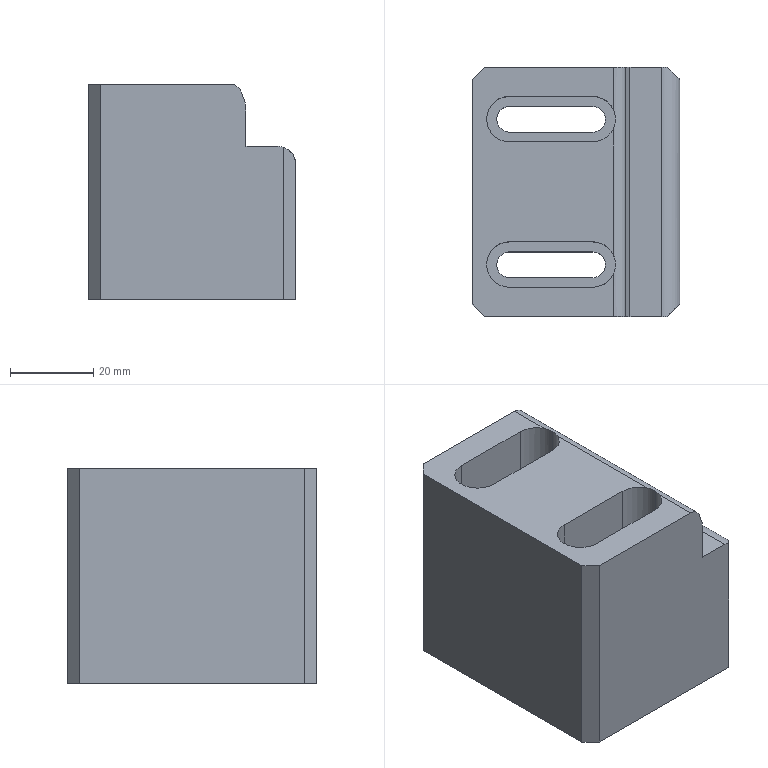Part | SolidWorks | features ICE 3, Chamfer 2, Fillet 2, Extrusion 1 | 1 solid | 38 faces | box 50 x 60 x 52 mm | volume 117515 mm3 | plane 23 | cylinder 15 | commonest cylinder face diameters 6.2 x6 11 x6 6 x2 8.8 x1
STEP:
#1=CARTESIAN_POINT('',(-2.536,-24.104,20.));
#2=VERTEX_POINT('',#1);
#3=CARTESIAN_POINT('',(-8.036,-18.604,20.));
#4=VERTEX_POINT('',#3);
#5=CARTESIAN_POINT('',(-8.036,-24.104,20.));
#6=DIRECTION('',(0.,0.,1.));
#7=DIRECTION('',(1.,0.,0.));
#8=AXIS2_PLACEMENT_3D('',#5,#6,#7);
#9=CIRCLE('',#8,5.5);
#10=EDGE_CURVE('',#2,#4,#9,.T.);
#11=ORIENTED_EDGE('',*,*,#10,.F.);
#12=CARTESIAN_POINT('',(-2.536,-24.104,51.97));
#13=VERTEX_POINT('',#12);
#14=CARTESIAN_POINT('',(-2.536,-24.104,20.));
#15=DIRECTION('',(0.,0.,1.));
#16=VECTOR('',#15,1000.);
#17=LINE('',#14,#16);
#18=EDGE_CURVE('',#2,#13,#17,.T.);
#19=ORIENTED_EDGE('',*,*,#18,.T.);
#20=CARTESIAN_POINT('',(-2.956,-21.995,52.));
#21=VERTEX_POINT('',#20);
#22=CARTESIAN_POINT('',(-2.536,-24.104,51.97));
#23=CARTESIAN_POINT('',(-2.536,-23.745,51.97));
#24=CARTESIAN_POINT('',(-2.57,-23.388,51.976));
#25=CARTESIAN_POINT('',(-2.711,-22.678,51.991));
#26=CARTESIAN_POINT('',(-2.817,-22.33,52.));
#27=CARTESIAN_POINT('',(-2.956,-21.995,52.));
#28=B_SPLINE_CURVE_WITH_KNOTS('',3,(#22,#23,#24,#25,#26,#27),.UNSPECIFIED.,.F.,.F.,(4,2,4),(0.002159,0.003239,0.004318),.UNSPECIFIED.);
#29=EDGE_CURVE('',#13,#21,#28,.T.);
#30=ORIENTED_EDGE('',*,*,#29,.T.);
#31=CARTESIAN_POINT('',(-8.036,-18.604,52.));
#32=VERTEX_POINT('',#31);
#33=CARTESIAN_POINT('',(-8.036,-24.104,52.));
#34=DIRECTION('',(0.,0.,1.));
#35=DIRECTION('',(1.,0.,0.));
#36=AXIS2_PLACEMENT_3D('',#33,#34,#35);
#37=CIRCLE('',#36,5.5);
#38=EDGE_CURVE('',#21,#32,#37,.T.);
#39=ORIENTED_EDGE('',*,*,#38,.T.);
#40=CARTESIAN_POINT('',(-8.036,-18.604,20.));
#41=DIRECTION('',(0.,0.,1.));
#42=VECTOR('',#41,1000.);
#43=LINE('',#40,#42);
#44=EDGE_CURVE('',#4,#32,#43,.T.);
#45=ORIENTED_EDGE('',*,*,#44,.F.);
#46=EDGE_LOOP('',(#11,#19,#30,#39,#45));
#47=FACE_OUTER_BOUND('',#46,.T.);
#48=CARTESIAN_POINT('',(-8.036,-24.104,20.));
#49=DIRECTION('',(0.,0.,1.));
#50=DIRECTION('',(1.,0.,0.));
#51=AXIS2_PLACEMENT_3D('',#48,#49,#50);
#52=CYLINDRICAL_SURFACE('',#51,5.5);
#53=ADVANCED_FACE('',(#47),#52,.F.);
#54=CARTESIAN_POINT('',(-2.536,10.896,20.));
#55=VERTEX_POINT('',#54);
#56=CARTESIAN_POINT('',(-8.036,16.396,20.));
#57=VERTEX_POINT('',#56);
#58=CARTESIAN_POINT('',(-8.036,10.896,20.));
#59=DIRECTION('',(0.,0.,1.));
#60=DIRECTION('',(1.,0.,0.));
#61=AXIS2_PLACEMENT_3D('',#58,#59,#60);
#62=CIRCLE('',#61,5.5);
#63=EDGE_CURVE('',#55,#57,#62,.T.);
#64=ORIENTED_EDGE('',*,*,#63,.F.);
#65=CARTESIAN_POINT('',(-2.536,10.896,51.97));
#66=VERTEX_POINT('',#65);
#67=CARTESIAN_POINT('',(-2.536,10.896,20.));
#68=DIRECTION('',(0.,0.,1.));
#69=VECTOR('',#68,1000.);
#70=LINE('',#67,#69);
#71=EDGE_CURVE('',#55,#66,#70,.T.);
#72=ORIENTED_EDGE('',*,*,#71,.T.);
#73=CARTESIAN_POINT('',(-2.956,13.005,52.));
#74=VERTEX_POINT('',#73);
#75=CARTESIAN_POINT('',(-2.536,10.896,51.97));
#76=CARTESIAN_POINT('',(-2.536,11.255,51.97));
#77=CARTESIAN_POINT('',(-2.57,11.612,51.976));
#78=CARTESIAN_POINT('',(-2.711,12.322,51.991));
#79=CARTESIAN_POINT('',(-2.817,12.67,52.));
#80=CARTESIAN_POINT('',(-2.956,13.005,52.));
#81=B_SPLINE_CURVE_WITH_KNOTS('',3,(#75,#76,#77,#78,#79,#80),.UNSPECIFIED.,.F.,.F.,(4,2,4),(0.002159,0.003239,0.004318),.UNSPECIFIED.);
#82=EDGE_CURVE('',#66,#74,#81,.T.);
#83=ORIENTED_EDGE('',*,*,#82,.T.);
#84=CARTESIAN_POINT('',(-8.036,16.396,52.));
#85=VERTEX_POINT('',#84);
#86=CARTESIAN_POINT('',(-8.036,10.896,52.));
#87=DIRECTION('',(0.,0.,1.));
#88=DIRECTION('',(1.,0.,0.));
#89=AXIS2_PLACEMENT_3D('',#86,#87,#88);
#90=CIRCLE('',#89,5.5);
#91=EDGE_CURVE('',#74,#85,#90,.T.);
#92=ORIENTED_EDGE('',*,*,#91,.T.);
#93=CARTESIAN_POINT('',(-8.036,16.396,20.));
#94=DIRECTION('',(0.,0.,1.));
#95=VECTOR('',#94,1000.);
#96=LINE('',#93,#95);
#97=EDGE_CURVE('',#57,#85,#96,.T.);
#98=ORIENTED_EDGE('',*,*,#97,.F.);
#99=EDGE_LOOP('',(#64,#72,#83,#92,#98));
#100=FACE_OUTER_BOUND('',#99,.T.);
#101=CARTESIAN_POINT('',(-8.036,10.896,20.));
#102=DIRECTION('',(0.,0.,1.));
#103=DIRECTION('',(1.,0.,0.));
#104=AXIS2_PLACEMENT_3D('',#101,#102,#103);
#105=CYLINDRICAL_SURFACE('',#104,5.5);
#106=ADVANCED_FACE('',(#100),#105,.F.);
#107=CARTESIAN_POINT('',(-4.936,10.896,0.));
#108=VERTEX_POINT('',#107);
#109=CARTESIAN_POINT('',(-8.036,13.996,0.));
#110=VERTEX_POINT('',#109);
#111=CARTESIAN_POINT('',(-8.036,10.896,0.));
#112=DIRECTION('',(0.,0.,1.));
#113=DIRECTION('',(1.,0.,0.));
#114=AXIS2_PLACEMENT_3D('',#111,#112,#113);
#115=CIRCLE('',#114,3.1);
#116=EDGE_CURVE('',#108,#110,#115,.T.);
#117=ORIENTED_EDGE('',*,*,#116,.F.);
#118=CARTESIAN_POINT('',(-4.936,10.896,20.));
#119=VERTEX_POINT('',#118);
#120=CARTESIAN_POINT('',(-4.936,10.896,0.));
#121=DIRECTION('',(0.,0.,1.));
#122=VECTOR('',#121,1000.);
#123=LINE('',#120,#122);
#124=EDGE_CURVE('',#108,#119,#123,.T.);
#125=ORIENTED_EDGE('',*,*,#124,.T.);
#126=CARTESIAN_POINT('',(-8.036,13.996,20.));
#127=VERTEX_POINT('',#126);
#128=CARTESIAN_POINT('',(-8.036,10.896,20.));
#129=DIRECTION('',(0.,0.,-1.));
#130=DIRECTION('',(1.,0.,0.));
#131=AXIS2_PLACEMENT_3D('',#128,#129,#130);
#132=CIRCLE('',#131,3.1);
#133=EDGE_CURVE('',#127,#119,#132,.T.);
#134=ORIENTED_EDGE('',*,*,#133,.F.);
#135=CARTESIAN_POINT('',(-8.036,13.996,0.));
#136=DIRECTION('',(0.,0.,1.));
#137=VECTOR('',#136,1000.);
#138=LINE('',#135,#137);
#139=EDGE_CURVE('',#110,#127,#138,.T.);
#140=ORIENTED_EDGE('',*,*,#139,.F.);
#141=EDGE_LOOP('',(#117,#125,#134,#140));
#142=FACE_OUTER_BOUND('',#141,.T.);
#143=CARTESIAN_POINT('',(-8.036,10.896,0.));
#144=DIRECTION('',(0.,0.,1.));
#145=DIRECTION('',(1.,0.,0.));
#146=AXIS2_PLACEMENT_3D('',#143,#144,#145);
#147=CYLINDRICAL_SURFACE('',#146,3.1);
#148=ADVANCED_FACE('',(#142),#147,.F.);
#149=CARTESIAN_POINT('',(-4.936,-24.104,0.));
#150=VERTEX_POINT('',#149);
#151=CARTESIAN_POINT('',(-8.036,-21.004,0.));
#152=VERTEX_POINT('',#151);
#153=CARTESIAN_POINT('',(-8.036,-24.104,0.));
#154=DIRECTION('',(0.,0.,1.));
#155=DIRECTION('',(1.,0.,0.));
#156=AXIS2_PLACEMENT_3D('',#153,#154,#155);
#157=CIRCLE('',#156,3.1);
#158=EDGE_CURVE('',#150,#152,#157,.T.);
#159=ORIENTED_EDGE('',*,*,#158,.F.);
#160=CARTESIAN_POINT('',(-4.936,-24.104,20.));
#161=VERTEX_POINT('',#160);
#162=CARTESIAN_POINT('',(-4.936,-24.104,0.));
#163=DIRECTION('',(0.,0.,1.));
#164=VECTOR('',#163,1000.);
#165=LINE('',#162,#164);
#166=EDGE_CURVE('',#150,#161,#165,.T.);
#167=ORIENTED_EDGE('',*,*,#166,.T.);
#168=CARTESIAN_POINT('',(-8.036,-21.004,20.));
#169=VERTEX_POINT('',#168);
#170=CARTESIAN_POINT('',(-8.036,-24.104,20.));
#171=DIRECTION('',(0.,0.,-1.));
#172=DIRECTION('',(1.,0.,0.));
#173=AXIS2_PLACEMENT_3D('',#170,#171,#172);
#174=CIRCLE('',#173,3.1);
#175=EDGE_CURVE('',#169,#161,#174,.T.);
#176=ORIENTED_EDGE('',*,*,#175,.F.);
#177=CARTESIAN_POINT('',(-8.036,-21.004,0.));
#178=DIRECTION('',(0.,0.,1.));
#179=VECTOR('',#178,1000.);
#180=LINE('',#177,#179);
#181=EDGE_CURVE('',#152,#169,#180,.T.);
#182=ORIENTED_EDGE('',*,*,#181,.F.);
#183=EDGE_LOOP('',(#159,#167,#176,#182));
#184=FACE_OUTER_BOUND('',#183,.T.);
#185=CARTESIAN_POINT('',(-8.036,-24.104,0.));
#186=DIRECTION('',(0.,0.,1.));
#187=DIRECTION('',(1.,0.,0.));
#188=AXIS2_PLACEMENT_3D('',#185,#186,#187);
#189=CYLINDRICAL_SURFACE('',#188,3.1);
#190=ADVANCED_FACE('',(#184),#189,.F.);
#191=CARTESIAN_POINT('',(-28.036,-27.204,20.));
#192=VERTEX_POINT('',#191);
#193=CARTESIAN_POINT('',(-28.036,-21.004,20.));
#194=VERTEX_POINT('',#193);
#195=CARTESIAN_POINT('',(-28.036,-24.104,20.));
#196=DIRECTION('',(0.,0.,-1.));
#197=DIRECTION('',(1.,0.,0.));
#198=AXIS2_PLACEMENT_3D('',#195,#196,#197);
#199=CIRCLE('',#198,3.1);
#200=EDGE_CURVE('',#192,#194,#199,.T.);
#201=ORIENTED_EDGE('',*,*,#200,.F.);
#202=CARTESIAN_POINT('',(-28.036,-27.204,0.));
#203=VERTEX_POINT('',#202);
#204=CARTESIAN_POINT('',(-28.036,-27.204,0.));
#205=DIRECTION('',(0.,0.,1.));
#206=VECTOR('',#205,1000.);
#207=LINE('',#204,#206);
#208=EDGE_CURVE('',#203,#192,#207,.T.);
#209=ORIENTED_EDGE('',*,*,#208,.F.);
#210=CARTESIAN_POINT('',(-28.036,-21.004,0.));
#211=VERTEX_POINT('',#210);
#212=CARTESIAN_POINT('',(-28.036,-24.104,0.));
#213=DIRECTION('',(0.,0.,1.));
#214=DIRECTION('',(1.,0.,0.));
#215=AXIS2_PLACEMENT_3D('',#212,#213,#214);
#216=CIRCLE('',#215,3.1);
#217=EDGE_CURVE('',#211,#203,#216,.T.);
#218=ORIENTED_EDGE('',*,*,#217,.F.);
#219=CARTESIAN_POINT('',(-28.036,-21.004,0.));
#220=DIRECTION('',(0.,0.,1.));
#221=VECTOR('',#220,1000.);
#222=LINE('',#219,#221);
#223=EDGE_CURVE('',#211,#194,#222,.T.);
#224=ORIENTED_EDGE('',*,*,#223,.T.);
#225=EDGE_LOOP('',(#201,#209,#218,#224));
#226=FACE_OUTER_BOUND('',#225,.T.);
#227=CARTESIAN_POINT('',(-28.036,-24.104,0.));
#228=DIRECTION('',(0.,0.,1.));
#229=DIRECTION('',(1.,0.,0.));
#230=AXIS2_PLACEMENT_3D('',#227,#228,#229);
#231=CYLINDRICAL_SURFACE('',#230,3.1);
#232=ADVANCED_FACE('',(#226),#231,.F.);
#233=CARTESIAN_POINT('',(-28.036,-21.004,20.));
#234=DIRECTION('',(1.,0.,0.));
#235=VECTOR('',#234,1000.);
#236=LINE('',#233,#235);
#237=EDGE_CURVE('',#194,#169,#236,.T.);
#238=ORIENTED_EDGE('',*,*,#237,.F.);
#239=ORIENTED_EDGE('',*,*,#223,.F.);
#240=CARTESIAN_POINT('',(-28.036,-21.004,0.));
#241=DIRECTION('',(-1.,0.,0.));
#242=VECTOR('',#241,1000.);
#243=LINE('',#240,#242);
#244=EDGE_CURVE('',#152,#211,#243,.T.);
#245=ORIENTED_EDGE('',*,*,#244,.F.);
#246=ORIENTED_EDGE('',*,*,#181,.T.);
#247=EDGE_LOOP('',(#238,#239,#245,#246));
#248=FACE_OUTER_BOUND('',#247,.T.);
#249=CARTESIAN_POINT('',(-28.036,-21.004,0.));
#250=DIRECTION('',(0.,1.,0.));
#251=DIRECTION('',(-1.,0.,0.));
#252=AXIS2_PLACEMENT_3D('',#249,#250,#251);
#253=PLANE('',#252);
#254=ADVANCED_FACE('',(#248),#253,.F.);
#255=ORIENTED_EDGE('',*,*,#166,.F.);
#256=CARTESIAN_POINT('',(-8.036,-27.204,0.));
#257=VERTEX_POINT('',#256);
#258=CARTESIAN_POINT('',(-8.036,-24.104,0.));
#259=DIRECTION('',(0.,0.,1.));
#260=DIRECTION('',(1.,0.,0.));
#261=AXIS2_PLACEMENT_3D('',#258,#259,#260);
#262=CIRCLE('',#261,3.1);
#263=EDGE_CURVE('',#257,#150,#262,.T.);
#264=ORIENTED_EDGE('',*,*,#263,.F.);
#265=CARTESIAN_POINT('',(-8.036,-27.204,20.));
#266=VERTEX_POINT('',#265);
#267=CARTESIAN_POINT('',(-8.036,-27.204,0.));
#268=DIRECTION('',(0.,0.,1.));
#269=VECTOR('',#268,1000.);
#270=LINE('',#267,#269);
#271=EDGE_CURVE('',#257,#266,#270,.T.);
#272=ORIENTED_EDGE('',*,*,#271,.T.);
#273=CARTESIAN_POINT('',(-8.036,-24.104,20.));
#274=DIRECTION('',(0.,0.,-1.));
#275=DIRECTION('',(1.,0.,0.));
#276=AXIS2_PLACEMENT_3D('',#273,#274,#275);
#277=CIRCLE('',#276,3.1);
#278=EDGE_CURVE('',#161,#266,#277,.T.);
#279=ORIENTED_EDGE('',*,*,#278,.F.);
#280=EDGE_LOOP('',(#255,#264,#272,#279));
#281=FACE_OUTER_BOUND('',#280,.T.);
#282=CARTESIAN_POINT('',(-8.036,-24.104,0.));
#283=DIRECTION('',(0.,0.,1.));
#284=DIRECTION('',(1.,0.,0.));
#285=AXIS2_PLACEMENT_3D('',#282,#283,#284);
#286=CYLINDRICAL_SURFACE('',#285,3.1);
#287=ADVANCED_FACE('',(#281),#286,.F.);
#288=CARTESIAN_POINT('',(-28.036,-27.204,20.));
#289=DIRECTION('',(-1.,0.,0.));
#290=VECTOR('',#289,1000.);
#291=LINE('',#288,#290);
#292=EDGE_CURVE('',#266,#192,#291,.T.);
#293=ORIENTED_EDGE('',*,*,#292,.F.);
#294=ORIENTED_EDGE('',*,*,#271,.F.);
#295=CARTESIAN_POINT('',(-28.036,-27.204,0.));
#296=DIRECTION('',(1.,0.,0.));
#297=VECTOR('',#296,1000.);
#298=LINE('',#295,#297);
#299=EDGE_CURVE('',#203,#257,#298,.T.);
#300=ORIENTED_EDGE('',*,*,#299,.F.);
#301=ORIENTED_EDGE('',*,*,#208,.T.);
#302=EDGE_LOOP('',(#293,#294,#300,#301));
#303=FACE_OUTER_BOUND('',#302,.T.);
#304=CARTESIAN_POINT('',(-28.036,-27.204,0.));
#305=DIRECTION('',(0.,-1.,0.));
#306=DIRECTION('',(1.,0.,0.));
#307=AXIS2_PLACEMENT_3D('',#304,#305,#306);
#308=PLANE('',#307);
#309=ADVANCED_FACE('',(#303),#308,.F.);
#310=CARTESIAN_POINT('',(-28.036,7.796,20.));
#311=VERTEX_POINT('',#310);
#312=CARTESIAN_POINT('',(-28.036,13.996,20.));
#313=VERTEX_POINT('',#312);
#314=CARTESIAN_POINT('',(-28.036,10.896,20.));
#315=DIRECTION('',(0.,0.,-1.));
#316=DIRECTION('',(1.,0.,0.));
#317=AXIS2_PLACEMENT_3D('',#314,#315,#316);
#318=CIRCLE('',#317,3.1);
#319=EDGE_CURVE('',#311,#313,#318,.T.);
#320=ORIENTED_EDGE('',*,*,#319,.F.);
#321=CARTESIAN_POINT('',(-28.036,7.796,0.));
#322=VERTEX_POINT('',#321);
#323=CARTESIAN_POINT('',(-28.036,7.796,0.));
#324=DIRECTION('',(0.,0.,1.));
#325=VECTOR('',#324,1000.);
#326=LINE('',#323,#325);
#327=EDGE_CURVE('',#322,#311,#326,.T.);
#328=ORIENTED_EDGE('',*,*,#327,.F.);
#329=CARTESIAN_POINT('',(-28.036,13.996,0.));
#330=VERTEX_POINT('',#329);
#331=CARTESIAN_POINT('',(-28.036,10.896,0.));
#332=DIRECTION('',(0.,0.,1.));
#333=DIRECTION('',(1.,0.,0.));
#334=AXIS2_PLACEMENT_3D('',#331,#332,#333);
#335=CIRCLE('',#334,3.1);
#336=EDGE_CURVE('',#330,#322,#335,.T.);
#337=ORIENTED_EDGE('',*,*,#336,.F.);
#338=CARTESIAN_POINT('',(-28.036,13.996,0.));
#339=DIRECTION('',(0.,0.,1.));
#340=VECTOR('',#339,1000.);
#341=LINE('',#338,#340);
#342=EDGE_CURVE('',#330,#313,#341,.T.);
#343=ORIENTED_EDGE('',*,*,#342,.T.);
#344=EDGE_LOOP('',(#320,#328,#337,#343));
#345=FACE_OUTER_BOUND('',#344,.T.);
#346=CARTESIAN_POINT('',(-28.036,10.896,0.));
#347=DIRECTION('',(0.,0.,1.));
#348=DIRECTION('',(1.,0.,0.));
#349=AXIS2_PLACEMENT_3D('',#346,#347,#348);
#350=CYLINDRICAL_SURFACE('',#349,3.1);
#351=ADVANCED_FACE('',(#345),#350,.F.);
#352=CARTESIAN_POINT('',(-28.036,13.996,20.));
#353=DIRECTION('',(1.,0.,0.));
#354=VECTOR('',#353,1000.);
#355=LINE('',#352,#354);
#356=EDGE_CURVE('',#313,#127,#355,.T.);
#357=ORIENTED_EDGE('',*,*,#356,.F.);
#358=ORIENTED_EDGE('',*,*,#342,.F.);
#359=CARTESIAN_POINT('',(-28.036,13.996,0.));
#360=DIRECTION('',(-1.,0.,0.));
#361=VECTOR('',#360,1000.);
#362=LINE('',#359,#361);
#363=EDGE_CURVE('',#110,#330,#362,.T.);
#364=ORIENTED_EDGE('',*,*,#363,.F.);
#365=ORIENTED_EDGE('',*,*,#139,.T.);
#366=EDGE_LOOP('',(#357,#358,#364,#365));
#367=FACE_OUTER_BOUND('',#366,.T.);
#368=CARTESIAN_POINT('',(-28.036,13.996,0.));
#369=DIRECTION('',(0.,1.,0.));
#370=DIRECTION('',(-1.,0.,0.));
#371=AXIS2_PLACEMENT_3D('',#368,#369,#370);
#372=PLANE('',#371);
#373=ADVANCED_FACE('',(#367),#372,.F.);
#374=ORIENTED_EDGE('',*,*,#124,.F.);
#375=CARTESIAN_POINT('',(-8.036,7.796,0.));
#376=VERTEX_POINT('',#375);
#377=CARTESIAN_POINT('',(-8.036,10.896,0.));
#378=DIRECTION('',(0.,0.,1.));
#379=DIRECTION('',(1.,0.,0.));
#380=AXIS2_PLACEMENT_3D('',#377,#378,#379);
#381=CIRCLE('',#380,3.1);
#382=EDGE_CURVE('',#376,#108,#381,.T.);
#383=ORIENTED_EDGE('',*,*,#382,.F.);
#384=CARTESIAN_POINT('',(-8.036,7.796,20.));
#385=VERTEX_POINT('',#384);
#386=CARTESIAN_POINT('',(-8.036,7.796,0.));
#387=DIRECTION('',(0.,0.,1.));
#388=VECTOR('',#387,1000.);
#389=LINE('',#386,#388);
#390=EDGE_CURVE('',#376,#385,#389,.T.);
#391=ORIENTED_EDGE('',*,*,#390,.T.);
#392=CARTESIAN_POINT('',(-8.036,10.896,20.));
#393=DIRECTION('',(0.,0.,-1.));
#394=DIRECTION('',(1.,0.,0.));
#395=AXIS2_PLACEMENT_3D('',#392,#393,#394);
#396=CIRCLE('',#395,3.1);
#397=EDGE_CURVE('',#119,#385,#396,.T.);
#398=ORIENTED_EDGE('',*,*,#397,.F.);
#399=EDGE_LOOP('',(#374,#383,#391,#398));
#400=FACE_OUTER_BOUND('',#399,.T.);
#401=CARTESIAN_POINT('',(-8.036,10.896,0.));
#402=DIRECTION('',(0.,0.,1.));
#403=DIRECTION('',(1.,0.,0.));
#404=AXIS2_PLACEMENT_3D('',#401,#402,#403);
#405=CYLINDRICAL_SURFACE('',#404,3.1);
#406=ADVANCED_FACE('',(#400),#405,.F.);
#407=CARTESIAN_POINT('',(-28.036,7.796,20.));
#408=DIRECTION('',(-1.,0.,0.));
#409=VECTOR('',#408,1000.);
#410=LINE('',#407,#409);
#411=EDGE_CURVE('',#385,#311,#410,.T.);
#412=ORIENTED_EDGE('',*,*,#411,.F.);
#413=ORIENTED_EDGE('',*,*,#390,.F.);
#414=CARTESIAN_POINT('',(-28.036,7.796,0.));
#415=DIRECTION('',(1.,0.,0.));
#416=VECTOR('',#415,1000.);
#417=LINE('',#414,#416);
#418=EDGE_CURVE('',#322,#376,#417,.T.);
#419=ORIENTED_EDGE('',*,*,#418,.F.);
#420=ORIENTED_EDGE('',*,*,#327,.T.);
#421=EDGE_LOOP('',(#412,#413,#419,#420));
#422=FACE_OUTER_BOUND('',#421,.T.);
#423=CARTESIAN_POINT('',(-28.036,7.796,0.));
#424=DIRECTION('',(0.,-1.,0.));
#425=DIRECTION('',(1.,0.,0.));
#426=AXIS2_PLACEMENT_3D('',#423,#424,#425);
#427=PLANE('',#426);
#428=ADVANCED_FACE('',(#422),#427,.F.);
#429=CARTESIAN_POINT('',(-37.036,20.396,52.));
#430=VERTEX_POINT('',#429);
#431=CARTESIAN_POINT('',(-37.036,-33.604,52.));
#432=VERTEX_POINT('',#431);
#433=CARTESIAN_POINT('',(-37.036,23.396,52.));
#434=DIRECTION('',(0.,-1.,0.));
#435=VECTOR('',#434,1000.);
#436=LINE('',#433,#435);
#437=EDGE_CURVE('',#430,#432,#436,.T.);
#438=ORIENTED_EDGE('',*,*,#437,.F.);
#439=CARTESIAN_POINT('',(-37.036,20.396,0.));
#440=VERTEX_POINT('',#439);
#441=CARTESIAN_POINT('',(-37.036,20.396,52.));
#442=DIRECTION('',(0.,0.,-1.));
#443=VECTOR('',#442,1000.);
#444=LINE('',#441,#443);
#445=EDGE_CURVE('',#430,#440,#444,.T.);
#446=ORIENTED_EDGE('',*,*,#445,.T.);
#447=CARTESIAN_POINT('',(-37.036,-33.604,0.));
#448=VERTEX_POINT('',#447);
#449=CARTESIAN_POINT('',(-37.036,23.396,0.));
#450=DIRECTION('',(0.,-1.,0.));
#451=VECTOR('',#450,1000.);
#452=LINE('',#449,#451);
#453=EDGE_CURVE('',#440,#448,#452,.T.);
#454=ORIENTED_EDGE('',*,*,#453,.T.);
#455=CARTESIAN_POINT('',(-37.036,-33.604,52.));
#456=DIRECTION('',(0.,0.,1.));
#457=VECTOR('',#456,1000.);
#458=LINE('',#455,#457);
#459=EDGE_CURVE('',#448,#432,#458,.T.);
#460=ORIENTED_EDGE('',*,*,#459,.T.);
#461=EDGE_LOOP('',(#438,#446,#454,#460));
#462=FACE_OUTER_BOUND('',#461,.T.);
#463=CARTESIAN_POINT('',(-37.036,23.396,52.));
#464=DIRECTION('',(1.,0.,0.));
#465=DIRECTION('',(0.,0.,-1.));
#466=AXIS2_PLACEMENT_3D('',#463,#464,#465);
#467=PLANE('',#466);
#468=ADVANCED_FACE('',(#462),#467,.F.);
#469=CARTESIAN_POINT('',(9.964,-36.604,0.));
#470=VERTEX_POINT('',#469);
#471=CARTESIAN_POINT('',(9.964,-36.604,36.771));
#472=VERTEX_POINT('',#471);
#473=CARTESIAN_POINT('',(9.964,-36.604,52.));
#474=DIRECTION('',(0.,0.,1.));
#475=VECTOR('',#474,1000.);
#476=LINE('',#473,#475);
#477=EDGE_CURVE('',#470,#472,#476,.T.);
#478=ORIENTED_EDGE('',*,*,#477,.T.);
#479=CARTESIAN_POINT('',(8.564,-36.604,37.));
#480=VERTEX_POINT('',#479);
#481=CARTESIAN_POINT('',(8.564,-36.604,32.6));
#482=DIRECTION('',(0.,-1.,0.));
#483=DIRECTION('',(0.,0.,1.));
#484=AXIS2_PLACEMENT_3D('',#481,#482,#483);
#485=CIRCLE('',#484,4.4);
#486=EDGE_CURVE('',#472,#480,#485,.T.);
#487=ORIENTED_EDGE('',*,*,#486,.T.);
#488=CARTESIAN_POINT('',(0.9643,-36.604,37.));
#489=VERTEX_POINT('',#488);
#490=CARTESIAN_POINT('',(12.964,-36.604,37.));
#491=DIRECTION('',(1.,0.,0.));
#492=VECTOR('',#491,1000.);
#493=LINE('',#490,#492);
#494=EDGE_CURVE('',#489,#480,#493,.T.);
#495=ORIENTED_EDGE('',*,*,#494,.F.);
#496=CARTESIAN_POINT('',(0.9643,-36.604,46.471));
#497=VERTEX_POINT('',#496);
#498=CARTESIAN_POINT('',(0.9643,-36.604,37.));
#499=DIRECTION('',(0.,0.,1.));
#500=VECTOR('',#499,1000.);
#501=LINE('',#498,#500);
#502=EDGE_CURVE('',#489,#497,#501,.T.);
#503=ORIENTED_EDGE('',*,*,#502,.T.);
#504=CARTESIAN_POINT('',(0.7833,-36.604,47.497));
#505=VERTEX_POINT('',#504);
#506=CARTESIAN_POINT('',(-2.036,-36.604,46.471));
#507=DIRECTION('',(0.,-1.,0.));
#508=DIRECTION('',(0.,0.,1.));
#509=AXIS2_PLACEMENT_3D('',#506,#507,#508);
#510=CIRCLE('',#509,3.);
#511=EDGE_CURVE('',#497,#505,#510,.T.);
#512=ORIENTED_EDGE('',*,*,#511,.T.);
#513=CARTESIAN_POINT('',(-0.1371,-36.604,50.026));
#514=VERTEX_POINT('',#513);
#515=CARTESIAN_POINT('',(0.9643,-36.604,47.));
#516=DIRECTION('',(-0.342,0.,0.9397));
#517=VECTOR('',#516,1000.);
#518=LINE('',#515,#517);
#519=EDGE_CURVE('',#505,#514,#518,.T.);
#520=ORIENTED_EDGE('',*,*,#519,.T.);
#521=CARTESIAN_POINT('',(-2.956,-36.604,52.));
#522=VERTEX_POINT('',#521);
#523=CARTESIAN_POINT('',(-2.956,-36.604,49.));
#524=DIRECTION('',(0.,-1.,0.));
#525=DIRECTION('',(0.,0.,1.));
#526=AXIS2_PLACEMENT_3D('',#523,#524,#525);
#527=CIRCLE('',#526,3.);
#528=EDGE_CURVE('',#514,#522,#527,.T.);
#529=ORIENTED_EDGE('',*,*,#528,.T.);
#530=CARTESIAN_POINT('',(-34.036,-36.604,52.));
#531=VERTEX_POINT('',#530);
#532=CARTESIAN_POINT('',(-37.036,-36.604,52.));
#533=DIRECTION('',(1.,0.,0.));
#534=VECTOR('',#533,1000.);
#535=LINE('',#532,#534);
#536=EDGE_CURVE('',#531,#522,#535,.T.);
#537=ORIENTED_EDGE('',*,*,#536,.F.);
#538=CARTESIAN_POINT('',(-34.036,-36.604,0.));
#539=VERTEX_POINT('',#538);
#540=CARTESIAN_POINT('',(-34.036,-36.604,52.));
#541=DIRECTION('',(0.,0.,-1.));
#542=VECTOR('',#541,1000.);
#543=LINE('',#540,#542);
#544=EDGE_CURVE('',#531,#539,#543,.T.);
#545=ORIENTED_EDGE('',*,*,#544,.T.);
#546=CARTESIAN_POINT('',(-37.036,-36.604,0.));
#547=DIRECTION('',(1.,0.,0.));
#548=VECTOR('',#547,1000.);
#549=LINE('',#546,#548);
#550=EDGE_CURVE('',#539,#470,#549,.T.);
#551=ORIENTED_EDGE('',*,*,#550,.T.);
#552=EDGE_LOOP('',(#478,#487,#495,#503,#512,#520,#529,#537,#545,#551));
#553=FACE_OUTER_BOUND('',#552,.T.);
#554=CARTESIAN_POINT('',(-37.036,-36.604,52.));
#555=DIRECTION('',(0.,1.,0.));
#556=DIRECTION('',(0.,0.,1.));
#557=AXIS2_PLACEMENT_3D('',#554,#555,#556);
#558=PLANE('',#557);
#559=ADVANCED_FACE('',(#553),#558,.F.);
#560=CARTESIAN_POINT('',(12.964,20.396,0.));
#561=VERTEX_POINT('',#560);
#562=CARTESIAN_POINT('',(12.964,20.396,32.6));
#563=VERTEX_POINT('',#562);
#564=CARTESIAN_POINT('',(12.964,20.396,52.));
#565=DIRECTION('',(0.,0.,1.));
#566=VECTOR('',#565,1000.);
#567=LINE('',#564,#566);
#568=EDGE_CURVE('',#561,#563,#567,.T.);
#569=ORIENTED_EDGE('',*,*,#568,.T.);
#570=CARTESIAN_POINT('',(12.964,-33.604,32.6));
#571=VERTEX_POINT('',#570);
#572=CARTESIAN_POINT('',(12.964,23.396,32.6));
#573=DIRECTION('',(0.,-1.,0.));
#574=VECTOR('',#573,1000.);
#575=LINE('',#572,#574);
#576=EDGE_CURVE('',#563,#571,#575,.T.);
#577=ORIENTED_EDGE('',*,*,#576,.T.);
#578=CARTESIAN_POINT('',(12.964,-33.604,0.));
#579=VERTEX_POINT('',#578);
#580=CARTESIAN_POINT('',(12.964,-33.604,52.));
#581=DIRECTION('',(0.,0.,-1.));
#582=VECTOR('',#581,1000.);
#583=LINE('',#580,#582);
#584=EDGE_CURVE('',#571,#579,#583,.T.);
#585=ORIENTED_EDGE('',*,*,#584,.T.);
#586=CARTESIAN_POINT('',(12.964,23.396,0.));
#587=DIRECTION('',(0.,1.,0.));
#588=VECTOR('',#587,1000.);
#589=LINE('',#586,#588);
#590=EDGE_CURVE('',#579,#561,#589,.T.);
#591=ORIENTED_EDGE('',*,*,#590,.T.);
#592=EDGE_LOOP('',(#569,#577,#585,#591));
#593=FACE_OUTER_BOUND('',#592,.T.);
#594=CARTESIAN_POINT('',(12.964,23.396,52.));
#595=DIRECTION('',(-1.,0.,0.));
#596=DIRECTION('',(0.,-1.,0.));
#597=AXIS2_PLACEMENT_3D('',#594,#595,#596);
#598=PLANE('',#597);
#599=ADVANCED_FACE('',(#593),#598,.F.);
#600=CARTESIAN_POINT('',(8.564,23.396,37.));
#601=VERTEX_POINT('',#600);
#602=CARTESIAN_POINT('',(0.9643,23.396,37.));
#603=VERTEX_POINT('',#602);
#604=CARTESIAN_POINT('',(12.964,23.396,37.));
#605=DIRECTION('',(-1.,0.,0.));
#606=VECTOR('',#605,1000.);
#607=LINE('',#604,#606);
#608=EDGE_CURVE('',#601,#603,#607,.T.);
#609=ORIENTED_EDGE('',*,*,#608,.F.);
#610=CARTESIAN_POINT('',(9.964,23.396,36.771));
#611=VERTEX_POINT('',#610);
#612=CARTESIAN_POINT('',(8.564,23.396,32.6));
#613=DIRECTION('',(0.,1.,0.));
#614=DIRECTION('',(0.,0.,-1.));
#615=AXIS2_PLACEMENT_3D('',#612,#613,#614);
#616=CIRCLE('',#615,4.4);
#617=EDGE_CURVE('',#601,#611,#616,.T.);
#618=ORIENTED_EDGE('',*,*,#617,.T.);
#619=CARTESIAN_POINT('',(9.964,23.396,0.));
#620=VERTEX_POINT('',#619);
#621=CARTESIAN_POINT('',(9.964,23.396,52.));
#622=DIRECTION('',(0.,0.,-1.));
#623=VECTOR('',#622,1000.);
#624=LINE('',#621,#623);
#625=EDGE_CURVE('',#611,#620,#624,.T.);
#626=ORIENTED_EDGE('',*,*,#625,.T.);
#627=CARTESIAN_POINT('',(-34.036,23.396,0.));
#628=VERTEX_POINT('',#627);
#629=CARTESIAN_POINT('',(-37.036,23.396,0.));
#630=DIRECTION('',(-1.,0.,0.));
#631=VECTOR('',#630,1000.);
#632=LINE('',#629,#631);
#633=EDGE_CURVE('',#620,#628,#632,.T.);
#634=ORIENTED_EDGE('',*,*,#633,.T.);
#635=CARTESIAN_POINT('',(-34.036,23.396,52.));
#636=VERTEX_POINT('',#635);
#637=CARTESIAN_POINT('',(-34.036,23.396,52.));
#638=DIRECTION('',(0.,0.,1.));
#639=VECTOR('',#638,1000.);
#640=LINE('',#637,#639);
#641=EDGE_CURVE('',#628,#636,#640,.T.);
#642=ORIENTED_EDGE('',*,*,#641,.T.);
#643=CARTESIAN_POINT('',(-2.956,23.396,52.));
#644=VERTEX_POINT('',#643);
#645=CARTESIAN_POINT('',(-37.036,23.396,52.));
#646=DIRECTION('',(-1.,0.,0.));
#647=VECTOR('',#646,1000.);
#648=LINE('',#645,#647);
#649=EDGE_CURVE('',#644,#636,#648,.T.);
#650=ORIENTED_EDGE('',*,*,#649,.F.);
#651=CARTESIAN_POINT('',(-0.1371,23.396,50.026));
#652=VERTEX_POINT('',#651);
#653=CARTESIAN_POINT('',(-2.956,23.396,49.));
#654=DIRECTION('',(0.,1.,0.));
#655=DIRECTION('',(0.,0.,-1.));
#656=AXIS2_PLACEMENT_3D('',#653,#654,#655);
#657=CIRCLE('',#656,3.);
#658=EDGE_CURVE('',#644,#652,#657,.T.);
#659=ORIENTED_EDGE('',*,*,#658,.T.);
#660=CARTESIAN_POINT('',(0.7833,23.396,47.497));
#661=VERTEX_POINT('',#660);
#662=CARTESIAN_POINT('',(0.9643,23.396,47.));
#663=DIRECTION('',(0.342,0.,-0.9397));
#664=VECTOR('',#663,1000.);
#665=LINE('',#662,#664);
#666=EDGE_CURVE('',#652,#661,#665,.T.);
#667=ORIENTED_EDGE('',*,*,#666,.T.);
#668=CARTESIAN_POINT('',(0.9643,23.396,46.471));
#669=VERTEX_POINT('',#668);
#670=CARTESIAN_POINT('',(-2.036,23.396,46.471));
#671=DIRECTION('',(0.,1.,0.));
#672=DIRECTION('',(0.,0.,-1.));
#673=AXIS2_PLACEMENT_3D('',#670,#671,#672);
#674=CIRCLE('',#673,3.);
#675=EDGE_CURVE('',#661,#669,#674,.T.);
#676=ORIENTED_EDGE('',*,*,#675,.T.);
#677=CARTESIAN_POINT('',(0.9643,23.396,37.));
#678=DIRECTION('',(0.,0.,1.));
#679=VECTOR('',#678,1000.);
#680=LINE('',#677,#679);
#681=EDGE_CURVE('',#603,#669,#680,.T.);
#682=ORIENTED_EDGE('',*,*,#681,.F.);
#683=EDGE_LOOP('',(#609,#618,#626,#634,#642,#650,#659,#667,#676,#682));
#684=FACE_OUTER_BOUND('',#683,.T.);
#685=CARTESIAN_POINT('',(-37.036,23.396,52.));
#686=DIRECTION('',(0.,-1.,0.));
#687=DIRECTION('',(0.,0.,-1.));
#688=AXIS2_PLACEMENT_3D('',#685,#686,#687);
#689=PLANE('',#688);
#690=ADVANCED_FACE('',(#684),#689,.F.);
#691=ORIENTED_EDGE('',*,*,#536,.T.);
#692=CARTESIAN_POINT('',(-2.956,-26.213,52.));
#693=VERTEX_POINT('',#692);
#694=CARTESIAN_POINT('',(-2.956,0.,52.));
#695=DIRECTION('',(0.,1.,0.));
#696=VECTOR('',#695,1000.);
#697=LINE('',#694,#696);
#698=EDGE_CURVE('',#522,#693,#697,.T.);
#699=ORIENTED_EDGE('',*,*,#698,.T.);
#700=CARTESIAN_POINT('',(-8.036,-29.604,52.));
#701=VERTEX_POINT('',#700);
#702=CARTESIAN_POINT('',(-8.036,-24.104,52.));
#703=DIRECTION('',(0.,0.,1.));
#704=DIRECTION('',(1.,0.,0.));
#705=AXIS2_PLACEMENT_3D('',#702,#703,#704);
#706=CIRCLE('',#705,5.5);
#707=EDGE_CURVE('',#701,#693,#706,.T.);
#708=ORIENTED_EDGE('',*,*,#707,.F.);
#709=CARTESIAN_POINT('',(-28.036,-29.604,52.));
#710=VERTEX_POINT('',#709);
#711=CARTESIAN_POINT('',(-28.036,-29.604,52.));
#712=DIRECTION('',(1.,0.,0.));
#713=VECTOR('',#712,1000.);
#714=LINE('',#711,#713);
#715=EDGE_CURVE('',#710,#701,#714,.T.);
#716=ORIENTED_EDGE('',*,*,#715,.F.);
#717=CARTESIAN_POINT('',(-28.036,-18.604,52.));
#718=VERTEX_POINT('',#717);
#719=CARTESIAN_POINT('',(-28.036,-24.104,52.));
#720=DIRECTION('',(0.,0.,1.));
#721=DIRECTION('',(1.,0.,0.));
#722=AXIS2_PLACEMENT_3D('',#719,#720,#721);
#723=CIRCLE('',#722,5.5);
#724=EDGE_CURVE('',#718,#710,#723,.T.);
#725=ORIENTED_EDGE('',*,*,#724,.F.);
#726=CARTESIAN_POINT('',(-28.036,-18.604,52.));
#727=DIRECTION('',(-1.,0.,0.));
#728=VECTOR('',#727,1000.);
#729=LINE('',#726,#728);
#730=EDGE_CURVE('',#32,#718,#729,.T.);
#731=ORIENTED_EDGE('',*,*,#730,.F.);
#732=ORIENTED_EDGE('',*,*,#38,.F.);
#733=CARTESIAN_POINT('',(-2.956,8.787,52.));
#734=VERTEX_POINT('',#733);
#735=CARTESIAN_POINT('',(-2.956,0.,52.));
#736=DIRECTION('',(0.,1.,0.));
#737=VECTOR('',#736,1000.);
#738=LINE('',#735,#737);
#739=EDGE_CURVE('',#21,#734,#738,.T.);
#740=ORIENTED_EDGE('',*,*,#739,.T.);
#741=CARTESIAN_POINT('',(-8.036,5.396,52.));
#742=VERTEX_POINT('',#741);
#743=CARTESIAN_POINT('',(-8.036,10.896,52.));
#744=DIRECTION('',(0.,0.,1.));
#745=DIRECTION('',(1.,0.,0.));
#746=AXIS2_PLACEMENT_3D('',#743,#744,#745);
#747=CIRCLE('',#746,5.5);
#748=EDGE_CURVE('',#742,#734,#747,.T.);
#749=ORIENTED_EDGE('',*,*,#748,.F.);
#750=CARTESIAN_POINT('',(-28.036,5.396,52.));
#751=VERTEX_POINT('',#750);
#752=CARTESIAN_POINT('',(-28.036,5.396,52.));
#753=DIRECTION('',(1.,0.,0.));
#754=VECTOR('',#753,1000.);
#755=LINE('',#752,#754);
#756=EDGE_CURVE('',#751,#742,#755,.T.);
#757=ORIENTED_EDGE('',*,*,#756,.F.);
#758=CARTESIAN_POINT('',(-28.036,16.396,52.));
#759=VERTEX_POINT('',#758);
#760=CARTESIAN_POINT('',(-28.036,10.896,52.));
#761=DIRECTION('',(0.,0.,1.));
#762=DIRECTION('',(1.,0.,0.));
#763=AXIS2_PLACEMENT_3D('',#760,#761,#762);
#764=CIRCLE('',#763,5.5);
#765=EDGE_CURVE('',#759,#751,#764,.T.);
#766=ORIENTED_EDGE('',*,*,#765,.F.);
#767=CARTESIAN_POINT('',(-28.036,16.396,52.));
#768=DIRECTION('',(-1.,0.,0.));
#769=VECTOR('',#768,1000.);
#770=LINE('',#767,#769);
#771=EDGE_CURVE('',#85,#759,#770,.T.);
#772=ORIENTED_EDGE('',*,*,#771,.F.);
#773=ORIENTED_EDGE('',*,*,#91,.F.);
#774=CARTESIAN_POINT('',(-2.956,0.,52.));
#775=DIRECTION('',(0.,1.,0.));
#776=VECTOR('',#775,1000.);
#777=LINE('',#774,#776);
#778=EDGE_CURVE('',#74,#644,#777,.T.);
#779=ORIENTED_EDGE('',*,*,#778,.T.);
#780=ORIENTED_EDGE('',*,*,#649,.T.);
#781=CARTESIAN_POINT('',(-28.716,28.716,52.));
#782=DIRECTION('',(-0.7071,-0.7071,0.));
#783=VECTOR('',#782,1000.);
#784=LINE('',#781,#783);
#785=EDGE_CURVE('',#636,#430,#784,.T.);
#786=ORIENTED_EDGE('',*,*,#785,.T.);
#787=ORIENTED_EDGE('',*,*,#437,.T.);
#788=CARTESIAN_POINT('',(-35.32,-35.32,52.));
#789=DIRECTION('',(0.7071,-0.7071,0.));
#790=VECTOR('',#789,1000.);
#791=LINE('',#788,#790);
#792=EDGE_CURVE('',#432,#531,#791,.T.);
#793=ORIENTED_EDGE('',*,*,#792,.T.);
#794=EDGE_LOOP('',(#691,#699,#708,#716,#725,#731,#732,#740,#749,#757,#766,#772,#773,#779,#780,#786,#787,#793));
#795=FACE_OUTER_BOUND('',#794,.T.);
#796=CARTESIAN_POINT('',(0.,0.,52.));
#797=DIRECTION('',(0.,0.,1.));
#798=DIRECTION('',(1.,0.,0.));
#799=AXIS2_PLACEMENT_3D('',#796,#797,#798);
#800=PLANE('',#799);
#801=ADVANCED_FACE('',(#795),#800,.T.);
#802=ORIENTED_EDGE('',*,*,#244,.T.);
#803=ORIENTED_EDGE('',*,*,#217,.T.);
#804=ORIENTED_EDGE('',*,*,#299,.T.);
#805=ORIENTED_EDGE('',*,*,#263,.T.);
#806=ORIENTED_EDGE('',*,*,#158,.T.);
#807=EDGE_LOOP('',(#802,#803,#804,#805,#806));
#808=FACE_BOUND('',#807,.T.);
#809=ORIENTED_EDGE('',*,*,#363,.T.);
#810=ORIENTED_EDGE('',*,*,#336,.T.);
#811=ORIENTED_EDGE('',*,*,#418,.T.);
#812=ORIENTED_EDGE('',*,*,#382,.T.);
#813=ORIENTED_EDGE('',*,*,#116,.T.);
#814=EDGE_LOOP('',(#809,#810,#811,#812,#813));
#815=FACE_BOUND('',#814,.T.);
#816=ORIENTED_EDGE('',*,*,#633,.F.);
#817=CARTESIAN_POINT('',(9.964,23.396,0.));
#818=DIRECTION('',(0.7071,-0.7071,0.));
#819=VECTOR('',#818,1000.);
#820=LINE('',#817,#819);
#821=EDGE_CURVE('',#620,#561,#820,.T.);
#822=ORIENTED_EDGE('',*,*,#821,.T.);
#823=ORIENTED_EDGE('',*,*,#590,.F.);
#824=CARTESIAN_POINT('',(12.964,-33.604,0.));
#825=DIRECTION('',(-0.7071,-0.7071,0.));
#826=VECTOR('',#825,1000.);
#827=LINE('',#824,#826);
#828=EDGE_CURVE('',#579,#470,#827,.T.);
#829=ORIENTED_EDGE('',*,*,#828,.T.);
#830=ORIENTED_EDGE('',*,*,#550,.F.);
#831=CARTESIAN_POINT('',(-34.036,-36.604,0.));
#832=DIRECTION('',(-0.7071,0.7071,0.));
#833=VECTOR('',#832,1000.);
#834=LINE('',#831,#833);
#835=EDGE_CURVE('',#539,#448,#834,.T.);
#836=ORIENTED_EDGE('',*,*,#835,.T.);
#837=ORIENTED_EDGE('',*,*,#453,.F.);
#838=CARTESIAN_POINT('',(-37.036,20.396,0.));
#839=DIRECTION('',(0.7071,0.7071,0.));
#840=VECTOR('',#839,1000.);
#841=LINE('',#838,#840);
#842=EDGE_CURVE('',#440,#628,#841,.T.);
#843=ORIENTED_EDGE('',*,*,#842,.T.);
#844=EDGE_LOOP('',(#816,#822,#823,#829,#830,#836,#837,#843));
#845=FACE_OUTER_BOUND('',#844,.T.);
#846=CARTESIAN_POINT('',(0.,0.,0.));
#847=DIRECTION('',(0.,0.,1.));
#848=DIRECTION('',(1.,0.,0.));
#849=AXIS2_PLACEMENT_3D('',#846,#847,#848);
#850=PLANE('',#849);
#851=ADVANCED_FACE('',(#808,#815,#845),#850,.F.);
#852=ORIENTED_EDGE('',*,*,#681,.T.);
#853=CARTESIAN_POINT('',(0.9643,-36.604,46.471));
#854=DIRECTION('',(0.,-1.,0.));
#855=VECTOR('',#854,1000.);
#856=LINE('',#853,#855);
#857=EDGE_CURVE('',#669,#497,#856,.T.);
#858=ORIENTED_EDGE('',*,*,#857,.T.);
#859=ORIENTED_EDGE('',*,*,#502,.F.);
#860=CARTESIAN_POINT('',(0.9643,23.396,37.));
#861=DIRECTION('',(0.,-1.,0.));
#862=VECTOR('',#861,1000.);
#863=LINE('',#860,#862);
#864=EDGE_CURVE('',#603,#489,#863,.T.);
#865=ORIENTED_EDGE('',*,*,#864,.F.);
#866=EDGE_LOOP('',(#852,#858,#859,#865));
#867=FACE_OUTER_BOUND('',#866,.T.);
#868=CARTESIAN_POINT('',(0.9643,23.396,37.));
#869=DIRECTION('',(-1.,0.,0.));
#870=DIRECTION('',(0.,-1.,0.));
#871=AXIS2_PLACEMENT_3D('',#868,#869,#870);
#872=PLANE('',#871);
#873=ADVANCED_FACE('',(#867),#872,.F.);
#874=ORIENTED_EDGE('',*,*,#494,.T.);
#875=CARTESIAN_POINT('',(8.564,0.,37.));
#876=DIRECTION('',(0.,1.,0.));
#877=VECTOR('',#876,1000.);
#878=LINE('',#875,#877);
#879=EDGE_CURVE('',#480,#601,#878,.T.);
#880=ORIENTED_EDGE('',*,*,#879,.T.);
#881=ORIENTED_EDGE('',*,*,#608,.T.);
#882=ORIENTED_EDGE('',*,*,#864,.T.);
#883=EDGE_LOOP('',(#874,#880,#881,#882));
#884=FACE_OUTER_BOUND('',#883,.T.);
#885=CARTESIAN_POINT('',(0.,0.,37.));
#886=DIRECTION('',(0.,0.,-1.));
#887=DIRECTION('',(-1.,0.,0.));
#888=AXIS2_PLACEMENT_3D('',#885,#886,#887);
#889=PLANE('',#888);
#890=ADVANCED_FACE('',(#884),#889,.F.);
#891=CARTESIAN_POINT('',(-28.036,16.396,20.));
#892=VERTEX_POINT('',#891);
#893=CARTESIAN_POINT('',(-28.036,5.396,20.));
#894=VERTEX_POINT('',#893);
#895=CARTESIAN_POINT('',(-28.036,10.896,20.));
#896=DIRECTION('',(0.,0.,1.));
#897=DIRECTION('',(1.,0.,0.));
#898=AXIS2_PLACEMENT_3D('',#895,#896,#897);
#899=CIRCLE('',#898,5.5);
#900=EDGE_CURVE('',#892,#894,#899,.T.);
#901=ORIENTED_EDGE('',*,*,#900,.T.);
#902=CARTESIAN_POINT('',(-8.036,5.396,20.));
#903=VERTEX_POINT('',#902);
#904=CARTESIAN_POINT('',(-28.036,5.396,20.));
#905=DIRECTION('',(1.,0.,0.));
#906=VECTOR('',#905,1000.);
#907=LINE('',#904,#906);
#908=EDGE_CURVE('',#894,#903,#907,.T.);
#909=ORIENTED_EDGE('',*,*,#908,.T.);
#910=CARTESIAN_POINT('',(-8.036,10.896,20.));
#911=DIRECTION('',(0.,0.,1.));
#912=DIRECTION('',(1.,0.,0.));
#913=AXIS2_PLACEMENT_3D('',#910,#911,#912);
#914=CIRCLE('',#913,5.5);
#915=EDGE_CURVE('',#903,#55,#914,.T.);
#916=ORIENTED_EDGE('',*,*,#915,.T.);
#917=ORIENTED_EDGE('',*,*,#63,.T.);
#918=CARTESIAN_POINT('',(-28.036,16.396,20.));
#919=DIRECTION('',(-1.,0.,0.));
#920=VECTOR('',#919,1000.);
#921=LINE('',#918,#920);
#922=EDGE_CURVE('',#57,#892,#921,.T.);
#923=ORIENTED_EDGE('',*,*,#922,.T.);
#924=EDGE_LOOP('',(#901,#909,#916,#917,#923));
#925=FACE_OUTER_BOUND('',#924,.T.);
#926=ORIENTED_EDGE('',*,*,#319,.T.);
#927=ORIENTED_EDGE('',*,*,#356,.T.);
#928=ORIENTED_EDGE('',*,*,#133,.T.);
#929=ORIENTED_EDGE('',*,*,#397,.T.);
#930=ORIENTED_EDGE('',*,*,#411,.T.);
#931=EDGE_LOOP('',(#926,#927,#928,#929,#930));
#932=FACE_BOUND('',#931,.T.);
#933=CARTESIAN_POINT('',(-28.036,10.896,20.));
#934=DIRECTION('',(0.,0.,1.));
#935=DIRECTION('',(1.,0.,0.));
#936=AXIS2_PLACEMENT_3D('',#933,#934,#935);
#937=PLANE('',#936);
#938=ADVANCED_FACE('',(#925,#932),#937,.T.);
#939=ORIENTED_EDGE('',*,*,#765,.T.);
#940=CARTESIAN_POINT('',(-28.036,5.396,20.));
#941=DIRECTION('',(0.,0.,1.));
#942=VECTOR('',#941,1000.);
#943=LINE('',#940,#942);
#944=EDGE_CURVE('',#894,#751,#943,.T.);
#945=ORIENTED_EDGE('',*,*,#944,.F.);
#946=ORIENTED_EDGE('',*,*,#900,.F.);
#947=CARTESIAN_POINT('',(-28.036,16.396,20.));
#948=DIRECTION('',(0.,0.,1.));
#949=VECTOR('',#948,1000.);
#950=LINE('',#947,#949);
#951=EDGE_CURVE('',#892,#759,#950,.T.);
#952=ORIENTED_EDGE('',*,*,#951,.T.);
#953=EDGE_LOOP('',(#939,#945,#946,#952));
#954=FACE_OUTER_BOUND('',#953,.T.);
#955=CARTESIAN_POINT('',(-28.036,10.896,20.));
#956=DIRECTION('',(0.,0.,1.));
#957=DIRECTION('',(1.,0.,0.));
#958=AXIS2_PLACEMENT_3D('',#955,#956,#957);
#959=CYLINDRICAL_SURFACE('',#958,5.5);
#960=ADVANCED_FACE('',(#954),#959,.F.);
#961=ORIENTED_EDGE('',*,*,#771,.T.);
#962=ORIENTED_EDGE('',*,*,#951,.F.);
#963=ORIENTED_EDGE('',*,*,#922,.F.);
#964=ORIENTED_EDGE('',*,*,#97,.T.);
#965=EDGE_LOOP('',(#961,#962,#963,#964));
#966=FACE_OUTER_BOUND('',#965,.T.);
#967=CARTESIAN_POINT('',(-28.036,16.396,20.));
#968=DIRECTION('',(0.,1.,0.));
#969=DIRECTION('',(0.,0.,1.));
#970=AXIS2_PLACEMENT_3D('',#967,#968,#969);
#971=PLANE('',#970);
#972=ADVANCED_FACE('',(#966),#971,.F.);
#973=ORIENTED_EDGE('',*,*,#71,.F.);
#974=ORIENTED_EDGE('',*,*,#915,.F.);
#975=CARTESIAN_POINT('',(-8.036,5.396,20.));
#976=DIRECTION('',(0.,0.,1.));
#977=VECTOR('',#976,1000.);
#978=LINE('',#975,#977);
#979=EDGE_CURVE('',#903,#742,#978,.T.);
#980=ORIENTED_EDGE('',*,*,#979,.T.);
#981=ORIENTED_EDGE('',*,*,#748,.T.);
#982=CARTESIAN_POINT('',(-2.956,8.787,52.));
#983=CARTESIAN_POINT('',(-2.817,9.123,52.));
#984=CARTESIAN_POINT('',(-2.712,9.467,51.991));
#985=CARTESIAN_POINT('',(-2.571,10.174,51.976));
#986=CARTESIAN_POINT('',(-2.536,10.538,51.97));
#987=CARTESIAN_POINT('',(-2.536,10.896,51.97));
#988=B_SPLINE_CURVE_WITH_KNOTS('',3,(#982,#983,#984,#985,#986,#987),.UNSPECIFIED.,.F.,.F.,(4,2,4),(0.,0.001079,0.002159),.UNSPECIFIED.);
#989=EDGE_CURVE('',#734,#66,#988,.T.);
#990=ORIENTED_EDGE('',*,*,#989,.T.);
#991=EDGE_LOOP('',(#973,#974,#980,#981,#990));
#992=FACE_OUTER_BOUND('',#991,.T.);
#993=CARTESIAN_POINT('',(-8.036,10.896,20.));
#994=DIRECTION('',(0.,0.,1.));
#995=DIRECTION('',(1.,0.,0.));
#996=AXIS2_PLACEMENT_3D('',#993,#994,#995);
#997=CYLINDRICAL_SURFACE('',#996,5.5);
#998=ADVANCED_FACE('',(#992),#997,.F.);
#999=ORIENTED_EDGE('',*,*,#756,.T.);
#1000=ORIENTED_EDGE('',*,*,#979,.F.);
#1001=ORIENTED_EDGE('',*,*,#908,.F.);
#1002=ORIENTED_EDGE('',*,*,#944,.T.);
#1003=EDGE_LOOP('',(#999,#1000,#1001,#1002));
#1004=FACE_OUTER_BOUND('',#1003,.T.);
#1005=CARTESIAN_POINT('',(-28.036,5.396,20.));
#1006=DIRECTION('',(0.,-1.,0.));
#1007=DIRECTION('',(0.,0.,-1.));
#1008=AXIS2_PLACEMENT_3D('',#1005,#1006,#1007);
#1009=PLANE('',#1008);
#1010=ADVANCED_FACE('',(#1004),#1009,.F.);
#1011=CARTESIAN_POINT('',(-28.036,-18.604,20.));
#1012=VERTEX_POINT('',#1011);
#1013=CARTESIAN_POINT('',(-28.036,-29.604,20.));
#1014=VERTEX_POINT('',#1013);
#1015=CARTESIAN_POINT('',(-28.036,-24.104,20.));
#1016=DIRECTION('',(0.,0.,1.));
#1017=DIRECTION('',(1.,0.,0.));
#1018=AXIS2_PLACEMENT_3D('',#1015,#1016,#1017);
#1019=CIRCLE('',#1018,5.5);
#1020=EDGE_CURVE('',#1012,#1014,#1019,.T.);
#1021=ORIENTED_EDGE('',*,*,#1020,.T.);
#1022=CARTESIAN_POINT('',(-8.036,-29.604,20.));
#1023=VERTEX_POINT('',#1022);
#1024=CARTESIAN_POINT('',(-28.036,-29.604,20.));
#1025=DIRECTION('',(1.,0.,0.));
#1026=VECTOR('',#1025,1000.);
#1027=LINE('',#1024,#1026);
#1028=EDGE_CURVE('',#1014,#1023,#1027,.T.);
#1029=ORIENTED_EDGE('',*,*,#1028,.T.);
#1030=CARTESIAN_POINT('',(-8.036,-24.104,20.));
#1031=DIRECTION('',(0.,0.,1.));
#1032=DIRECTION('',(1.,0.,0.));
#1033=AXIS2_PLACEMENT_3D('',#1030,#1031,#1032);
#1034=CIRCLE('',#1033,5.5);
#1035=EDGE_CURVE('',#1023,#2,#1034,.T.);
#1036=ORIENTED_EDGE('',*,*,#1035,.T.);
#1037=ORIENTED_EDGE('',*,*,#10,.T.);
#1038=CARTESIAN_POINT('',(-28.036,-18.604,20.));
#1039=DIRECTION('',(-1.,0.,0.));
#1040=VECTOR('',#1039,1000.);
#1041=LINE('',#1038,#1040);
#1042=EDGE_CURVE('',#4,#1012,#1041,.T.);
#1043=ORIENTED_EDGE('',*,*,#1042,.T.);
#1044=EDGE_LOOP('',(#1021,#1029,#1036,#1037,#1043));
#1045=FACE_OUTER_BOUND('',#1044,.T.);
#1046=ORIENTED_EDGE('',*,*,#200,.T.);
#1047=ORIENTED_EDGE('',*,*,#237,.T.);
#1048=ORIENTED_EDGE('',*,*,#175,.T.);
#1049=ORIENTED_EDGE('',*,*,#278,.T.);
#1050=ORIENTED_EDGE('',*,*,#292,.T.);
#1051=EDGE_LOOP('',(#1046,#1047,#1048,#1049,#1050));
#1052=FACE_BOUND('',#1051,.T.);
#1053=CARTESIAN_POINT('',(-28.036,-24.104,20.));
#1054=DIRECTION('',(0.,0.,1.));
#1055=DIRECTION('',(1.,0.,0.));
#1056=AXIS2_PLACEMENT_3D('',#1053,#1054,#1055);
#1057=PLANE('',#1056);
#1058=ADVANCED_FACE('',(#1045,#1052),#1057,.T.);
#1059=ORIENTED_EDGE('',*,*,#724,.T.);
#1060=CARTESIAN_POINT('',(-28.036,-29.604,20.));
#1061=DIRECTION('',(0.,0.,1.));
#1062=VECTOR('',#1061,1000.);
#1063=LINE('',#1060,#1062);
#1064=EDGE_CURVE('',#1014,#710,#1063,.T.);
#1065=ORIENTED_EDGE('',*,*,#1064,.F.);
#1066=ORIENTED_EDGE('',*,*,#1020,.F.);
#1067=CARTESIAN_POINT('',(-28.036,-18.604,20.));
#1068=DIRECTION('',(0.,0.,1.));
#1069=VECTOR('',#1068,1000.);
#1070=LINE('',#1067,#1069);
#1071=EDGE_CURVE('',#1012,#718,#1070,.T.);
#1072=ORIENTED_EDGE('',*,*,#1071,.T.);
#1073=EDGE_LOOP('',(#1059,#1065,#1066,#1072));
#1074=FACE_OUTER_BOUND('',#1073,.T.);
#1075=CARTESIAN_POINT('',(-28.036,-24.104,20.));
#1076=DIRECTION('',(0.,0.,1.));
#1077=DIRECTION('',(1.,0.,0.));
#1078=AXIS2_PLACEMENT_3D('',#1075,#1076,#1077);
#1079=CYLINDRICAL_SURFACE('',#1078,5.5);
#1080=ADVANCED_FACE('',(#1074),#1079,.F.);
#1081=ORIENTED_EDGE('',*,*,#730,.T.);
#1082=ORIENTED_EDGE('',*,*,#1071,.F.);
#1083=ORIENTED_EDGE('',*,*,#1042,.F.);
#1084=ORIENTED_EDGE('',*,*,#44,.T.);
#1085=EDGE_LOOP('',(#1081,#1082,#1083,#1084));
#1086=FACE_OUTER_BOUND('',#1085,.T.);
#1087=CARTESIAN_POINT('',(-28.036,-18.604,20.));
#1088=DIRECTION('',(0.,1.,0.));
#1089=DIRECTION('',(0.,0.,1.));
#1090=AXIS2_PLACEMENT_3D('',#1087,#1088,#1089);
#1091=PLANE('',#1090);
#1092=ADVANCED_FACE('',(#1086),#1091,.F.);
#1093=ORIENTED_EDGE('',*,*,#18,.F.);
#1094=ORIENTED_EDGE('',*,*,#1035,.F.);
#1095=CARTESIAN_POINT('',(-8.036,-29.604,20.));
#1096=DIRECTION('',(0.,0.,1.));
#1097=VECTOR('',#1096,1000.);
#1098=LINE('',#1095,#1097);
#1099=EDGE_CURVE('',#1023,#701,#1098,.T.);
#1100=ORIENTED_EDGE('',*,*,#1099,.T.);
#1101=ORIENTED_EDGE('',*,*,#707,.T.);
#1102=CARTESIAN_POINT('',(-2.956,-26.213,52.));
#1103=CARTESIAN_POINT('',(-2.817,-25.877,52.));
#1104=CARTESIAN_POINT('',(-2.712,-25.533,51.991));
#1105=CARTESIAN_POINT('',(-2.571,-24.826,51.976));
#1106=CARTESIAN_POINT('',(-2.536,-24.462,51.97));
#1107=CARTESIAN_POINT('',(-2.536,-24.104,51.97));
#1108=B_SPLINE_CURVE_WITH_KNOTS('',3,(#1102,#1103,#1104,#1105,#1106,#1107),.UNSPECIFIED.,.F.,.F.,(4,2,4),(0.,0.001079,0.002159),.UNSPECIFIED.);
#1109=EDGE_CURVE('',#693,#13,#1108,.T.);
#1110=ORIENTED_EDGE('',*,*,#1109,.T.);
#1111=EDGE_LOOP('',(#1093,#1094,#1100,#1101,#1110));
#1112=FACE_OUTER_BOUND('',#1111,.T.);
#1113=CARTESIAN_POINT('',(-8.036,-24.104,20.));
#1114=DIRECTION('',(0.,0.,1.));
#1115=DIRECTION('',(1.,0.,0.));
#1116=AXIS2_PLACEMENT_3D('',#1113,#1114,#1115);
#1117=CYLINDRICAL_SURFACE('',#1116,5.5);
#1118=ADVANCED_FACE('',(#1112),#1117,.F.);
#1119=ORIENTED_EDGE('',*,*,#715,.T.);
#1120=ORIENTED_EDGE('',*,*,#1099,.F.);
#1121=ORIENTED_EDGE('',*,*,#1028,.F.);
#1122=ORIENTED_EDGE('',*,*,#1064,.T.);
#1123=EDGE_LOOP('',(#1119,#1120,#1121,#1122));
#1124=FACE_OUTER_BOUND('',#1123,.T.);
#1125=CARTESIAN_POINT('',(-28.036,-29.604,20.));
#1126=DIRECTION('',(0.,-1.,0.));
#1127=DIRECTION('',(0.,0.,-1.));
#1128=AXIS2_PLACEMENT_3D('',#1125,#1126,#1127);
#1129=PLANE('',#1128);
#1130=ADVANCED_FACE('',(#1124),#1129,.F.);
#1131=ORIENTED_EDGE('',*,*,#625,.F.);
#1132=CARTESIAN_POINT('',(9.964,23.396,36.771));
#1133=CARTESIAN_POINT('',(11.821,21.54,36.148));
#1134=CARTESIAN_POINT('',(12.964,20.396,34.558));
#1135=CARTESIAN_POINT('',(12.964,20.396,32.6));
#1136=(BOUNDED_CURVE()B_SPLINE_CURVE(3,(#1132,#1133,#1134,#1135),.UNSPECIFIED.,.F.,.F.)B_SPLINE_CURVE_WITH_KNOTS((4,4),(1.895,3.142),.UNSPECIFIED.)CURVE()GEOMETRIC_REPRESENTATION_ITEM()RATIONAL_B_SPLINE_CURVE((1.,0.8746,0.8746,1.))REPRESENTATION_ITEM(''));
#1137=EDGE_CURVE('',#611,#563,#1136,.T.);
#1138=ORIENTED_EDGE('',*,*,#1137,.T.);
#1139=ORIENTED_EDGE('',*,*,#568,.F.);
#1140=ORIENTED_EDGE('',*,*,#821,.F.);
#1141=EDGE_LOOP('',(#1131,#1138,#1139,#1140));
#1142=FACE_OUTER_BOUND('',#1141,.T.);
#1143=CARTESIAN_POINT('',(9.964,23.396,52.));
#1144=DIRECTION('',(-0.7071,-0.7071,0.));
#1145=DIRECTION('',(0.,0.,-1.));
#1146=AXIS2_PLACEMENT_3D('',#1143,#1144,#1145);
#1147=PLANE('',#1146);
#1148=ADVANCED_FACE('',(#1142),#1147,.F.);
#1149=ORIENTED_EDGE('',*,*,#584,.F.);
#1150=CARTESIAN_POINT('',(12.964,-33.604,32.6));
#1151=CARTESIAN_POINT('',(12.964,-33.604,34.558));
#1152=CARTESIAN_POINT('',(11.821,-34.747,36.148));
#1153=CARTESIAN_POINT('',(9.964,-36.604,36.771));
#1154=(BOUNDED_CURVE()B_SPLINE_CURVE(3,(#1150,#1151,#1152,#1153),.UNSPECIFIED.,.F.,.F.)B_SPLINE_CURVE_WITH_KNOTS((4,4),(0.,1.247),.UNSPECIFIED.)CURVE()GEOMETRIC_REPRESENTATION_ITEM()RATIONAL_B_SPLINE_CURVE((1.,0.8746,0.8746,1.))REPRESENTATION_ITEM(''));
#1155=EDGE_CURVE('',#571,#472,#1154,.T.);
#1156=ORIENTED_EDGE('',*,*,#1155,.T.);
#1157=ORIENTED_EDGE('',*,*,#477,.F.);
#1158=ORIENTED_EDGE('',*,*,#828,.F.);
#1159=EDGE_LOOP('',(#1149,#1156,#1157,#1158));
#1160=FACE_OUTER_BOUND('',#1159,.T.);
#1161=CARTESIAN_POINT('',(12.964,-33.604,52.));
#1162=DIRECTION('',(-0.7071,0.7071,0.));
#1163=DIRECTION('',(0.,0.,-1.));
#1164=AXIS2_PLACEMENT_3D('',#1161,#1162,#1163);
#1165=PLANE('',#1164);
#1166=ADVANCED_FACE('',(#1160),#1165,.F.);
#1167=ORIENTED_EDGE('',*,*,#785,.F.);
#1168=ORIENTED_EDGE('',*,*,#641,.F.);
#1169=ORIENTED_EDGE('',*,*,#842,.F.);
#1170=ORIENTED_EDGE('',*,*,#445,.F.);
#1171=EDGE_LOOP('',(#1167,#1168,#1169,#1170));
#1172=FACE_OUTER_BOUND('',#1171,.T.);
#1173=CARTESIAN_POINT('',(-37.036,20.396,52.));
#1174=DIRECTION('',(0.7071,-0.7071,0.));
#1175=DIRECTION('',(0.,0.,-1.));
#1176=AXIS2_PLACEMENT_3D('',#1173,#1174,#1175);
#1177=PLANE('',#1176);
#1178=ADVANCED_FACE('',(#1172),#1177,.F.);
#1179=ORIENTED_EDGE('',*,*,#792,.F.);
#1180=ORIENTED_EDGE('',*,*,#459,.F.);
#1181=ORIENTED_EDGE('',*,*,#835,.F.);
#1182=ORIENTED_EDGE('',*,*,#544,.F.);
#1183=EDGE_LOOP('',(#1179,#1180,#1181,#1182));
#1184=FACE_OUTER_BOUND('',#1183,.T.);
#1185=CARTESIAN_POINT('',(-34.036,-36.604,52.));
#1186=DIRECTION('',(0.7071,0.7071,0.));
#1187=DIRECTION('',(0.,0.,-1.));
#1188=AXIS2_PLACEMENT_3D('',#1185,#1186,#1187);
#1189=PLANE('',#1188);
#1190=ADVANCED_FACE('',(#1184),#1189,.F.);
#1191=ORIENTED_EDGE('',*,*,#519,.F.);
#1192=CARTESIAN_POINT('',(0.7833,23.396,47.497));
#1193=DIRECTION('',(0.,1.,0.));
#1194=VECTOR('',#1193,1000.);
#1195=LINE('',#1192,#1194);
#1196=EDGE_CURVE('',#505,#661,#1195,.T.);
#1197=ORIENTED_EDGE('',*,*,#1196,.T.);
#1198=ORIENTED_EDGE('',*,*,#666,.F.);
#1199=CARTESIAN_POINT('',(-0.1371,23.396,50.026));
#1200=DIRECTION('',(0.,-1.,0.));
#1201=VECTOR('',#1200,1000.);
#1202=LINE('',#1199,#1201);
#1203=EDGE_CURVE('',#652,#514,#1202,.T.);
#1204=ORIENTED_EDGE('',*,*,#1203,.T.);
#1205=EDGE_LOOP('',(#1191,#1197,#1198,#1204));
#1206=FACE_OUTER_BOUND('',#1205,.T.);
#1207=CARTESIAN_POINT('',(0.9643,23.396,47.));
#1208=DIRECTION('',(0.9397,0.,0.342));
#1209=DIRECTION('',(0.,1.,0.));
#1210=AXIS2_PLACEMENT_3D('',#1207,#1208,#1209);
#1211=PLANE('',#1210);
#1212=ADVANCED_FACE('',(#1206),#1211,.T.);
#1213=ORIENTED_EDGE('',*,*,#675,.F.);
#1214=ORIENTED_EDGE('',*,*,#1196,.F.);
#1215=ORIENTED_EDGE('',*,*,#511,.F.);
#1216=ORIENTED_EDGE('',*,*,#857,.F.);
#1217=EDGE_LOOP('',(#1213,#1214,#1215,#1216));
#1218=FACE_OUTER_BOUND('',#1217,.T.);
#1219=CARTESIAN_POINT('',(-2.036,23.396,46.471));
#1220=DIRECTION('',(0.,1.,0.));
#1221=DIRECTION('',(-1.,0.,0.));
#1222=AXIS2_PLACEMENT_3D('',#1219,#1220,#1221);
#1223=CYLINDRICAL_SURFACE('',#1222,3.);
#1224=ADVANCED_FACE('',(#1218),#1223,.T.);
#1225=ORIENTED_EDGE('',*,*,#528,.F.);
#1226=ORIENTED_EDGE('',*,*,#1203,.F.);
#1227=ORIENTED_EDGE('',*,*,#658,.F.);
#1228=ORIENTED_EDGE('',*,*,#778,.F.);
#1229=ORIENTED_EDGE('',*,*,#82,.F.);
#1230=ORIENTED_EDGE('',*,*,#989,.F.);
#1231=ORIENTED_EDGE('',*,*,#739,.F.);
#1232=ORIENTED_EDGE('',*,*,#29,.F.);
#1233=ORIENTED_EDGE('',*,*,#1109,.F.);
#1234=ORIENTED_EDGE('',*,*,#698,.F.);
#1235=EDGE_LOOP('',(#1225,#1226,#1227,#1228,#1229,#1230,#1231,#1232,#1233,#1234));
#1236=FACE_OUTER_BOUND('',#1235,.T.);
#1237=CARTESIAN_POINT('',(-2.956,0.,49.));
#1238=DIRECTION('',(0.,1.,0.));
#1239=DIRECTION('',(-1.,0.,0.));
#1240=AXIS2_PLACEMENT_3D('',#1237,#1238,#1239);
#1241=CYLINDRICAL_SURFACE('',#1240,3.);
#1242=ADVANCED_FACE('',(#1236),#1241,.T.);
#1243=ORIENTED_EDGE('',*,*,#1155,.F.);
#1244=ORIENTED_EDGE('',*,*,#576,.F.);
#1245=ORIENTED_EDGE('',*,*,#1137,.F.);
#1246=ORIENTED_EDGE('',*,*,#617,.F.);
#1247=ORIENTED_EDGE('',*,*,#879,.F.);
#1248=ORIENTED_EDGE('',*,*,#486,.F.);
#1249=EDGE_LOOP('',(#1243,#1244,#1245,#1246,#1247,#1248));
#1250=FACE_OUTER_BOUND('',#1249,.T.);
#1251=CARTESIAN_POINT('',(8.564,0.,32.6));
#1252=DIRECTION('',(0.,1.,0.));
#1253=DIRECTION('',(-1.,0.,0.));
#1254=AXIS2_PLACEMENT_3D('',#1251,#1252,#1253);
#1255=CYLINDRICAL_SURFACE('',#1254,4.4);
#1256=ADVANCED_FACE('',(#1250),#1255,.T.);
#1257=CLOSED_SHELL('',(#53,#106,#148,#190,#232,#254,#287,#309,#351,#373,#406,#428,#468,#559,#599,#690,#801,#851,#873,#890,#938,#960,#972,#998,#1010,#1058,#1080,#1092,#1118,#1130,#1148,#1166,#1178,#1190,#1212,#1224,#1242,#1256));
#1258=MANIFOLD_SOLID_BREP('',#1257);
#1259=CARTESIAN_POINT('',(0.,0.,0.));
#1260=DIRECTION('',(0.,0.,1.));
#1261=DIRECTION('',(1.,0.,0.));
#1262=AXIS2_PLACEMENT_3D('',#1259,#1260,#1261);
#1263=(LENGTH_UNIT()NAMED_UNIT(*)SI_UNIT(.MILLI.,.METRE.));
#1264=UNCERTAINTY_MEASURE_WITH_UNIT(LENGTH_MEASURE(0.00001),#1263,'','');
#1265=(NAMED_UNIT(*)PLANE_ANGLE_UNIT()SI_UNIT($,.RADIAN.));
#1266=(NAMED_UNIT(*)SI_UNIT($,.STERADIAN.)SOLID_ANGLE_UNIT());
#1267=(GEOMETRIC_REPRESENTATION_CONTEXT(3)GLOBAL_UNCERTAINTY_ASSIGNED_CONTEXT((#1264))GLOBAL_UNIT_ASSIGNED_CONTEXT((#1263,#1265,#1266))REPRESENTATION_CONTEXT('',''));
#1268=ADVANCED_BREP_SHAPE_REPRESENTATION('',(#1258,#1262),#1267);